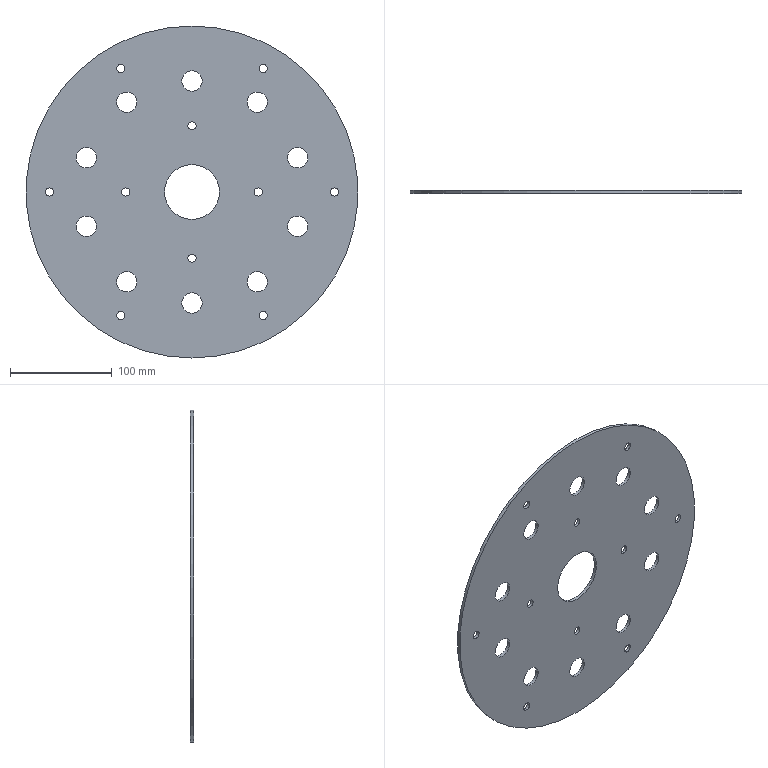Part | STEP file | JBJ-P-1012-03 | 1 solid | 24 faces | box 326 x 3 x 326 mm | volume 232604 mm3 | cylinder 22 | plane 2 | commonest cylinder face diameters 8 x10 20 x10 54 x1 326 x1
STEP:
#1=CARTESIAN_POINT('',(-140.,3.,4.));
#2=VERTEX_POINT('',#1);
#3=CARTESIAN_POINT('',(-140.,3.,0.));
#4=DIRECTION('',(0.,1.,0.));
#5=DIRECTION('',(0.,0.,1.));
#6=AXIS2_PLACEMENT_3D('',#3,#4,#5);
#7=CIRCLE('',#6,4.);
#8=EDGE_CURVE('',#2,#2,#7,.T.);
#9=ORIENTED_EDGE('',*,*,#8,.F.);
#10=EDGE_LOOP('',(#9));
#11=FACE_BOUND('',#10,.T.);
#12=CARTESIAN_POINT('',(-70.,3.,-117.244));
#13=VERTEX_POINT('',#12);
#14=CARTESIAN_POINT('',(-70.,3.,-121.244));
#15=DIRECTION('',(0.,1.,0.));
#16=DIRECTION('',(0.,0.,1.));
#17=AXIS2_PLACEMENT_3D('',#14,#15,#16);
#18=CIRCLE('',#17,4.);
#19=EDGE_CURVE('',#13,#13,#18,.T.);
#20=ORIENTED_EDGE('',*,*,#19,.F.);
#21=EDGE_LOOP('',(#20));
#22=FACE_BOUND('',#21,.T.);
#23=CARTESIAN_POINT('',(70.,3.,-117.244));
#24=VERTEX_POINT('',#23);
#25=CARTESIAN_POINT('',(70.,3.,-121.244));
#26=DIRECTION('',(0.,1.,0.));
#27=DIRECTION('',(0.,0.,1.));
#28=AXIS2_PLACEMENT_3D('',#25,#26,#27);
#29=CIRCLE('',#28,4.);
#30=EDGE_CURVE('',#24,#24,#29,.T.);
#31=ORIENTED_EDGE('',*,*,#30,.F.);
#32=EDGE_LOOP('',(#31));
#33=FACE_BOUND('',#32,.T.);
#34=CARTESIAN_POINT('',(140.,3.,4.));
#35=VERTEX_POINT('',#34);
#36=CARTESIAN_POINT('',(140.,3.,0.));
#37=DIRECTION('',(0.,1.,0.));
#38=DIRECTION('',(0.,0.,1.));
#39=AXIS2_PLACEMENT_3D('',#36,#37,#38);
#40=CIRCLE('',#39,4.);
#41=EDGE_CURVE('',#35,#35,#40,.T.);
#42=ORIENTED_EDGE('',*,*,#41,.F.);
#43=EDGE_LOOP('',(#42));
#44=FACE_BOUND('',#43,.T.);
#45=CARTESIAN_POINT('',(70.,3.,125.244));
#46=VERTEX_POINT('',#45);
#47=CARTESIAN_POINT('',(70.,3.,121.244));
#48=DIRECTION('',(0.,1.,0.));
#49=DIRECTION('',(0.,0.,1.));
#50=AXIS2_PLACEMENT_3D('',#47,#48,#49);
#51=CIRCLE('',#50,4.);
#52=EDGE_CURVE('',#46,#46,#51,.T.);
#53=ORIENTED_EDGE('',*,*,#52,.F.);
#54=EDGE_LOOP('',(#53));
#55=FACE_BOUND('',#54,.T.);
#56=CARTESIAN_POINT('',(-70.,3.,125.244));
#57=VERTEX_POINT('',#56);
#58=CARTESIAN_POINT('',(-70.,3.,121.244));
#59=DIRECTION('',(0.,1.,0.));
#60=DIRECTION('',(0.,0.,1.));
#61=AXIS2_PLACEMENT_3D('',#58,#59,#60);
#62=CIRCLE('',#61,4.);
#63=EDGE_CURVE('',#57,#57,#62,.T.);
#64=ORIENTED_EDGE('',*,*,#63,.F.);
#65=EDGE_LOOP('',(#64));
#66=FACE_BOUND('',#65,.T.);
#67=CARTESIAN_POINT('',(65.,3.,4.));
#68=VERTEX_POINT('',#67);
#69=CARTESIAN_POINT('',(65.,3.,0.));
#70=DIRECTION('',(0.,1.,0.));
#71=DIRECTION('',(0.,0.,1.));
#72=AXIS2_PLACEMENT_3D('',#69,#70,#71);
#73=CIRCLE('',#72,4.);
#74=EDGE_CURVE('',#68,#68,#73,.T.);
#75=ORIENTED_EDGE('',*,*,#74,.F.);
#76=EDGE_LOOP('',(#75));
#77=FACE_BOUND('',#76,.T.);
#78=CARTESIAN_POINT('',(0.,3.,-61.));
#79=VERTEX_POINT('',#78);
#80=CARTESIAN_POINT('',(0.,3.,-65.));
#81=DIRECTION('',(0.,1.,0.));
#82=DIRECTION('',(0.,0.,1.));
#83=AXIS2_PLACEMENT_3D('',#80,#81,#82);
#84=CIRCLE('',#83,4.);
#85=EDGE_CURVE('',#79,#79,#84,.T.);
#86=ORIENTED_EDGE('',*,*,#85,.F.);
#87=EDGE_LOOP('',(#86));
#88=FACE_BOUND('',#87,.T.);
#89=CARTESIAN_POINT('',(-65.,3.,4.));
#90=VERTEX_POINT('',#89);
#91=CARTESIAN_POINT('',(-65.,3.,0.));
#92=DIRECTION('',(0.,1.,0.));
#93=DIRECTION('',(0.,0.,1.));
#94=AXIS2_PLACEMENT_3D('',#91,#92,#93);
#95=CIRCLE('',#94,4.);
#96=EDGE_CURVE('',#90,#90,#95,.T.);
#97=ORIENTED_EDGE('',*,*,#96,.F.);
#98=EDGE_LOOP('',(#97));
#99=FACE_BOUND('',#98,.T.);
#100=CARTESIAN_POINT('',(0.,3.,69.));
#101=VERTEX_POINT('',#100);
#102=CARTESIAN_POINT('',(0.,3.,65.));
#103=DIRECTION('',(0.,1.,0.));
#104=DIRECTION('',(0.,0.,1.));
#105=AXIS2_PLACEMENT_3D('',#102,#103,#104);
#106=CIRCLE('',#105,4.);
#107=EDGE_CURVE('',#101,#101,#106,.T.);
#108=ORIENTED_EDGE('',*,*,#107,.F.);
#109=EDGE_LOOP('',(#108));
#110=FACE_BOUND('',#109,.T.);
#111=CARTESIAN_POINT('',(0.,3.,119.));
#112=VERTEX_POINT('',#111);
#113=CARTESIAN_POINT('',(0.,3.,109.));
#114=DIRECTION('',(0.,1.,0.));
#115=DIRECTION('',(0.,0.,1.));
#116=AXIS2_PLACEMENT_3D('',#113,#114,#115);
#117=CIRCLE('',#116,10.);
#118=EDGE_CURVE('',#112,#112,#117,.T.);
#119=ORIENTED_EDGE('',*,*,#118,.F.);
#120=EDGE_LOOP('',(#119));
#121=FACE_BOUND('',#120,.T.);
#122=CARTESIAN_POINT('',(103.665,3.,43.683));
#123=VERTEX_POINT('',#122);
#124=CARTESIAN_POINT('',(103.665,3.,33.683));
#125=DIRECTION('',(0.,1.,0.));
#126=DIRECTION('',(0.,0.,1.));
#127=AXIS2_PLACEMENT_3D('',#124,#125,#126);
#128=CIRCLE('',#127,10.);
#129=EDGE_CURVE('',#123,#123,#128,.T.);
#130=ORIENTED_EDGE('',*,*,#129,.F.);
#131=EDGE_LOOP('',(#130));
#132=FACE_BOUND('',#131,.T.);
#133=CARTESIAN_POINT('',(64.069,3.,-78.183));
#134=VERTEX_POINT('',#133);
#135=CARTESIAN_POINT('',(64.069,3.,-88.183));
#136=DIRECTION('',(0.,1.,0.));
#137=DIRECTION('',(0.,0.,1.));
#138=AXIS2_PLACEMENT_3D('',#135,#136,#137);
#139=CIRCLE('',#138,10.);
#140=EDGE_CURVE('',#134,#134,#139,.T.);
#141=ORIENTED_EDGE('',*,*,#140,.F.);
#142=EDGE_LOOP('',(#141));
#143=FACE_BOUND('',#142,.T.);
#144=CARTESIAN_POINT('',(-64.069,3.,-78.183));
#145=VERTEX_POINT('',#144);
#146=CARTESIAN_POINT('',(-64.069,3.,-88.183));
#147=DIRECTION('',(0.,1.,0.));
#148=DIRECTION('',(0.,0.,1.));
#149=AXIS2_PLACEMENT_3D('',#146,#147,#148);
#150=CIRCLE('',#149,10.);
#151=EDGE_CURVE('',#145,#145,#150,.T.);
#152=ORIENTED_EDGE('',*,*,#151,.F.);
#153=EDGE_LOOP('',(#152));
#154=FACE_BOUND('',#153,.T.);
#155=CARTESIAN_POINT('',(-103.665,3.,-23.683));
#156=VERTEX_POINT('',#155);
#157=CARTESIAN_POINT('',(-103.665,3.,-33.683));
#158=DIRECTION('',(0.,1.,0.));
#159=DIRECTION('',(0.,0.,1.));
#160=AXIS2_PLACEMENT_3D('',#157,#158,#159);
#161=CIRCLE('',#160,10.);
#162=EDGE_CURVE('',#156,#156,#161,.T.);
#163=ORIENTED_EDGE('',*,*,#162,.F.);
#164=EDGE_LOOP('',(#163));
#165=FACE_BOUND('',#164,.T.);
#166=CARTESIAN_POINT('',(0.,3.,163.));
#167=VERTEX_POINT('',#166);
#168=CARTESIAN_POINT('',(0.,3.,0.));
#169=DIRECTION('',(0.,1.,0.));
#170=DIRECTION('',(0.,0.,1.));
#171=AXIS2_PLACEMENT_3D('',#168,#169,#170);
#172=CIRCLE('',#171,163.);
#173=EDGE_CURVE('',#167,#167,#172,.T.);
#174=ORIENTED_EDGE('',*,*,#173,.T.);
#175=EDGE_LOOP('',(#174));
#176=FACE_OUTER_BOUND('',#175,.T.);
#177=CARTESIAN_POINT('',(0.,3.,27.));
#178=VERTEX_POINT('',#177);
#179=CARTESIAN_POINT('',(0.,3.,0.));
#180=DIRECTION('',(0.,1.,0.));
#181=DIRECTION('',(0.,0.,1.));
#182=AXIS2_PLACEMENT_3D('',#179,#180,#181);
#183=CIRCLE('',#182,27.);
#184=EDGE_CURVE('',#178,#178,#183,.T.);
#185=ORIENTED_EDGE('',*,*,#184,.F.);
#186=EDGE_LOOP('',(#185));
#187=FACE_BOUND('',#186,.T.);
#188=CARTESIAN_POINT('',(-103.665,3.,43.683));
#189=VERTEX_POINT('',#188);
#190=CARTESIAN_POINT('',(-103.665,3.,33.683));
#191=DIRECTION('',(0.,1.,0.));
#192=DIRECTION('',(0.,0.,1.));
#193=AXIS2_PLACEMENT_3D('',#190,#191,#192);
#194=CIRCLE('',#193,10.);
#195=EDGE_CURVE('',#189,#189,#194,.T.);
#196=ORIENTED_EDGE('',*,*,#195,.F.);
#197=EDGE_LOOP('',(#196));
#198=FACE_BOUND('',#197,.T.);
#199=CARTESIAN_POINT('',(0.,3.,-99.));
#200=VERTEX_POINT('',#199);
#201=CARTESIAN_POINT('',(0.,3.,-109.));
#202=DIRECTION('',(0.,1.,0.));
#203=DIRECTION('',(0.,0.,1.));
#204=AXIS2_PLACEMENT_3D('',#201,#202,#203);
#205=CIRCLE('',#204,10.);
#206=EDGE_CURVE('',#200,#200,#205,.T.);
#207=ORIENTED_EDGE('',*,*,#206,.F.);
#208=EDGE_LOOP('',(#207));
#209=FACE_BOUND('',#208,.T.);
#210=CARTESIAN_POINT('',(103.665,3.,-23.683));
#211=VERTEX_POINT('',#210);
#212=CARTESIAN_POINT('',(103.665,3.,-33.683));
#213=DIRECTION('',(0.,1.,0.));
#214=DIRECTION('',(0.,0.,1.));
#215=AXIS2_PLACEMENT_3D('',#212,#213,#214);
#216=CIRCLE('',#215,10.);
#217=EDGE_CURVE('',#211,#211,#216,.T.);
#218=ORIENTED_EDGE('',*,*,#217,.F.);
#219=EDGE_LOOP('',(#218));
#220=FACE_BOUND('',#219,.T.);
#221=CARTESIAN_POINT('',(64.069,3.,98.183));
#222=VERTEX_POINT('',#221);
#223=CARTESIAN_POINT('',(64.069,3.,88.183));
#224=DIRECTION('',(0.,1.,0.));
#225=DIRECTION('',(0.,0.,1.));
#226=AXIS2_PLACEMENT_3D('',#223,#224,#225);
#227=CIRCLE('',#226,10.);
#228=EDGE_CURVE('',#222,#222,#227,.T.);
#229=ORIENTED_EDGE('',*,*,#228,.F.);
#230=EDGE_LOOP('',(#229));
#231=FACE_BOUND('',#230,.T.);
#232=CARTESIAN_POINT('',(-64.069,3.,98.183));
#233=VERTEX_POINT('',#232);
#234=CARTESIAN_POINT('',(-64.069,3.,88.183));
#235=DIRECTION('',(0.,1.,0.));
#236=DIRECTION('',(0.,0.,1.));
#237=AXIS2_PLACEMENT_3D('',#234,#235,#236);
#238=CIRCLE('',#237,10.);
#239=EDGE_CURVE('',#233,#233,#238,.T.);
#240=ORIENTED_EDGE('',*,*,#239,.F.);
#241=EDGE_LOOP('',(#240));
#242=FACE_BOUND('',#241,.T.);
#243=CARTESIAN_POINT('',(0.,3.,0.));
#244=DIRECTION('',(0.,1.,0.));
#245=DIRECTION('',(0.,0.,1.));
#246=AXIS2_PLACEMENT_3D('',#243,#244,#245);
#247=PLANE('',#246);
#248=ADVANCED_FACE('',(#11,#22,#33,#44,#55,#66,#77,#88,#99,#110,#121,#132,#143,#154,#165,#176,#187,#198,#209,#220,#231,#242),#247,.T.);
#249=CARTESIAN_POINT('',(-140.,0.,4.));
#250=VERTEX_POINT('',#249);
#251=CARTESIAN_POINT('',(-140.,0.,0.));
#252=DIRECTION('',(0.,1.,0.));
#253=DIRECTION('',(0.,0.,1.));
#254=AXIS2_PLACEMENT_3D('',#251,#252,#253);
#255=CIRCLE('',#254,4.);
#256=EDGE_CURVE('',#250,#250,#255,.T.);
#257=ORIENTED_EDGE('',*,*,#256,.T.);
#258=EDGE_LOOP('',(#257));
#259=FACE_BOUND('',#258,.T.);
#260=CARTESIAN_POINT('',(-70.,0.,-117.244));
#261=VERTEX_POINT('',#260);
#262=CARTESIAN_POINT('',(-70.,0.,-121.244));
#263=DIRECTION('',(0.,1.,0.));
#264=DIRECTION('',(0.,0.,1.));
#265=AXIS2_PLACEMENT_3D('',#262,#263,#264);
#266=CIRCLE('',#265,4.);
#267=EDGE_CURVE('',#261,#261,#266,.T.);
#268=ORIENTED_EDGE('',*,*,#267,.T.);
#269=EDGE_LOOP('',(#268));
#270=FACE_BOUND('',#269,.T.);
#271=CARTESIAN_POINT('',(70.,0.,-117.244));
#272=VERTEX_POINT('',#271);
#273=CARTESIAN_POINT('',(70.,0.,-121.244));
#274=DIRECTION('',(0.,1.,0.));
#275=DIRECTION('',(0.,0.,1.));
#276=AXIS2_PLACEMENT_3D('',#273,#274,#275);
#277=CIRCLE('',#276,4.);
#278=EDGE_CURVE('',#272,#272,#277,.T.);
#279=ORIENTED_EDGE('',*,*,#278,.T.);
#280=EDGE_LOOP('',(#279));
#281=FACE_BOUND('',#280,.T.);
#282=CARTESIAN_POINT('',(140.,0.,4.));
#283=VERTEX_POINT('',#282);
#284=CARTESIAN_POINT('',(140.,0.,0.));
#285=DIRECTION('',(0.,1.,0.));
#286=DIRECTION('',(0.,0.,1.));
#287=AXIS2_PLACEMENT_3D('',#284,#285,#286);
#288=CIRCLE('',#287,4.);
#289=EDGE_CURVE('',#283,#283,#288,.T.);
#290=ORIENTED_EDGE('',*,*,#289,.T.);
#291=EDGE_LOOP('',(#290));
#292=FACE_BOUND('',#291,.T.);
#293=CARTESIAN_POINT('',(70.,0.,125.244));
#294=VERTEX_POINT('',#293);
#295=CARTESIAN_POINT('',(70.,0.,121.244));
#296=DIRECTION('',(0.,1.,0.));
#297=DIRECTION('',(0.,0.,1.));
#298=AXIS2_PLACEMENT_3D('',#295,#296,#297);
#299=CIRCLE('',#298,4.);
#300=EDGE_CURVE('',#294,#294,#299,.T.);
#301=ORIENTED_EDGE('',*,*,#300,.T.);
#302=EDGE_LOOP('',(#301));
#303=FACE_BOUND('',#302,.T.);
#304=CARTESIAN_POINT('',(-70.,0.,125.244));
#305=VERTEX_POINT('',#304);
#306=CARTESIAN_POINT('',(-70.,0.,121.244));
#307=DIRECTION('',(0.,1.,0.));
#308=DIRECTION('',(0.,0.,1.));
#309=AXIS2_PLACEMENT_3D('',#306,#307,#308);
#310=CIRCLE('',#309,4.);
#311=EDGE_CURVE('',#305,#305,#310,.T.);
#312=ORIENTED_EDGE('',*,*,#311,.T.);
#313=EDGE_LOOP('',(#312));
#314=FACE_BOUND('',#313,.T.);
#315=CARTESIAN_POINT('',(65.,0.,4.));
#316=VERTEX_POINT('',#315);
#317=CARTESIAN_POINT('',(65.,0.,0.));
#318=DIRECTION('',(0.,1.,0.));
#319=DIRECTION('',(0.,0.,1.));
#320=AXIS2_PLACEMENT_3D('',#317,#318,#319);
#321=CIRCLE('',#320,4.);
#322=EDGE_CURVE('',#316,#316,#321,.T.);
#323=ORIENTED_EDGE('',*,*,#322,.T.);
#324=EDGE_LOOP('',(#323));
#325=FACE_BOUND('',#324,.T.);
#326=CARTESIAN_POINT('',(0.,0.,-61.));
#327=VERTEX_POINT('',#326);
#328=CARTESIAN_POINT('',(0.,0.,-65.));
#329=DIRECTION('',(0.,1.,0.));
#330=DIRECTION('',(0.,0.,1.));
#331=AXIS2_PLACEMENT_3D('',#328,#329,#330);
#332=CIRCLE('',#331,4.);
#333=EDGE_CURVE('',#327,#327,#332,.T.);
#334=ORIENTED_EDGE('',*,*,#333,.T.);
#335=EDGE_LOOP('',(#334));
#336=FACE_BOUND('',#335,.T.);
#337=CARTESIAN_POINT('',(-65.,0.,4.));
#338=VERTEX_POINT('',#337);
#339=CARTESIAN_POINT('',(-65.,0.,0.));
#340=DIRECTION('',(0.,1.,0.));
#341=DIRECTION('',(0.,0.,1.));
#342=AXIS2_PLACEMENT_3D('',#339,#340,#341);
#343=CIRCLE('',#342,4.);
#344=EDGE_CURVE('',#338,#338,#343,.T.);
#345=ORIENTED_EDGE('',*,*,#344,.T.);
#346=EDGE_LOOP('',(#345));
#347=FACE_BOUND('',#346,.T.);
#348=CARTESIAN_POINT('',(0.,0.,69.));
#349=VERTEX_POINT('',#348);
#350=CARTESIAN_POINT('',(0.,0.,65.));
#351=DIRECTION('',(0.,1.,0.));
#352=DIRECTION('',(0.,0.,1.));
#353=AXIS2_PLACEMENT_3D('',#350,#351,#352);
#354=CIRCLE('',#353,4.);
#355=EDGE_CURVE('',#349,#349,#354,.T.);
#356=ORIENTED_EDGE('',*,*,#355,.T.);
#357=EDGE_LOOP('',(#356));
#358=FACE_BOUND('',#357,.T.);
#359=CARTESIAN_POINT('',(0.,0.,163.));
#360=VERTEX_POINT('',#359);
#361=CARTESIAN_POINT('',(0.,0.,0.));
#362=DIRECTION('',(0.,1.,0.));
#363=DIRECTION('',(0.,0.,1.));
#364=AXIS2_PLACEMENT_3D('',#361,#362,#363);
#365=CIRCLE('',#364,163.);
#366=EDGE_CURVE('',#360,#360,#365,.T.);
#367=ORIENTED_EDGE('',*,*,#366,.F.);
#368=EDGE_LOOP('',(#367));
#369=FACE_OUTER_BOUND('',#368,.T.);
#370=CARTESIAN_POINT('',(0.,0.,27.));
#371=VERTEX_POINT('',#370);
#372=CARTESIAN_POINT('',(0.,0.,0.));
#373=DIRECTION('',(0.,1.,0.));
#374=DIRECTION('',(0.,0.,1.));
#375=AXIS2_PLACEMENT_3D('',#372,#373,#374);
#376=CIRCLE('',#375,27.);
#377=EDGE_CURVE('',#371,#371,#376,.T.);
#378=ORIENTED_EDGE('',*,*,#377,.T.);
#379=EDGE_LOOP('',(#378));
#380=FACE_BOUND('',#379,.T.);
#381=CARTESIAN_POINT('',(-103.665,0.,-23.683));
#382=VERTEX_POINT('',#381);
#383=CARTESIAN_POINT('',(-103.665,0.,-33.683));
#384=DIRECTION('',(0.,1.,0.));
#385=DIRECTION('',(0.,0.,1.));
#386=AXIS2_PLACEMENT_3D('',#383,#384,#385);
#387=CIRCLE('',#386,10.);
#388=EDGE_CURVE('',#382,#382,#387,.T.);
#389=ORIENTED_EDGE('',*,*,#388,.T.);
#390=EDGE_LOOP('',(#389));
#391=FACE_BOUND('',#390,.T.);
#392=CARTESIAN_POINT('',(-103.665,0.,43.683));
#393=VERTEX_POINT('',#392);
#394=CARTESIAN_POINT('',(-103.665,0.,33.683));
#395=DIRECTION('',(0.,1.,0.));
#396=DIRECTION('',(0.,0.,1.));
#397=AXIS2_PLACEMENT_3D('',#394,#395,#396);
#398=CIRCLE('',#397,10.);
#399=EDGE_CURVE('',#393,#393,#398,.T.);
#400=ORIENTED_EDGE('',*,*,#399,.T.);
#401=EDGE_LOOP('',(#400));
#402=FACE_BOUND('',#401,.T.);
#403=CARTESIAN_POINT('',(-64.069,0.,-78.183));
#404=VERTEX_POINT('',#403);
#405=CARTESIAN_POINT('',(-64.069,0.,-88.183));
#406=DIRECTION('',(0.,1.,0.));
#407=DIRECTION('',(0.,0.,1.));
#408=AXIS2_PLACEMENT_3D('',#405,#406,#407);
#409=CIRCLE('',#408,10.);
#410=EDGE_CURVE('',#404,#404,#409,.T.);
#411=ORIENTED_EDGE('',*,*,#410,.T.);
#412=EDGE_LOOP('',(#411));
#413=FACE_BOUND('',#412,.T.);
#414=CARTESIAN_POINT('',(0.,0.,-99.));
#415=VERTEX_POINT('',#414);
#416=CARTESIAN_POINT('',(0.,0.,-109.));
#417=DIRECTION('',(0.,1.,0.));
#418=DIRECTION('',(0.,0.,1.));
#419=AXIS2_PLACEMENT_3D('',#416,#417,#418);
#420=CIRCLE('',#419,10.);
#421=EDGE_CURVE('',#415,#415,#420,.T.);
#422=ORIENTED_EDGE('',*,*,#421,.T.);
#423=EDGE_LOOP('',(#422));
#424=FACE_BOUND('',#423,.T.);
#425=CARTESIAN_POINT('',(64.069,0.,-78.183));
#426=VERTEX_POINT('',#425);
#427=CARTESIAN_POINT('',(64.069,0.,-88.183));
#428=DIRECTION('',(0.,1.,0.));
#429=DIRECTION('',(0.,0.,1.));
#430=AXIS2_PLACEMENT_3D('',#427,#428,#429);
#431=CIRCLE('',#430,10.);
#432=EDGE_CURVE('',#426,#426,#431,.T.);
#433=ORIENTED_EDGE('',*,*,#432,.T.);
#434=EDGE_LOOP('',(#433));
#435=FACE_BOUND('',#434,.T.);
#436=CARTESIAN_POINT('',(103.665,0.,-23.683));
#437=VERTEX_POINT('',#436);
#438=CARTESIAN_POINT('',(103.665,0.,-33.683));
#439=DIRECTION('',(0.,1.,0.));
#440=DIRECTION('',(0.,0.,1.));
#441=AXIS2_PLACEMENT_3D('',#438,#439,#440);
#442=CIRCLE('',#441,10.);
#443=EDGE_CURVE('',#437,#437,#442,.T.);
#444=ORIENTED_EDGE('',*,*,#443,.T.);
#445=EDGE_LOOP('',(#444));
#446=FACE_BOUND('',#445,.T.);
#447=CARTESIAN_POINT('',(103.665,0.,43.683));
#448=VERTEX_POINT('',#447);
#449=CARTESIAN_POINT('',(103.665,0.,33.683));
#450=DIRECTION('',(0.,1.,0.));
#451=DIRECTION('',(0.,0.,1.));
#452=AXIS2_PLACEMENT_3D('',#449,#450,#451);
#453=CIRCLE('',#452,10.);
#454=EDGE_CURVE('',#448,#448,#453,.T.);
#455=ORIENTED_EDGE('',*,*,#454,.T.);
#456=EDGE_LOOP('',(#455));
#457=FACE_BOUND('',#456,.T.);
#458=CARTESIAN_POINT('',(64.069,0.,98.183));
#459=VERTEX_POINT('',#458);
#460=CARTESIAN_POINT('',(64.069,0.,88.183));
#461=DIRECTION('',(0.,1.,0.));
#462=DIRECTION('',(0.,0.,1.));
#463=AXIS2_PLACEMENT_3D('',#460,#461,#462);
#464=CIRCLE('',#463,10.);
#465=EDGE_CURVE('',#459,#459,#464,.T.);
#466=ORIENTED_EDGE('',*,*,#465,.T.);
#467=EDGE_LOOP('',(#466));
#468=FACE_BOUND('',#467,.T.);
#469=CARTESIAN_POINT('',(0.,0.,119.));
#470=VERTEX_POINT('',#469);
#471=CARTESIAN_POINT('',(0.,0.,109.));
#472=DIRECTION('',(0.,1.,0.));
#473=DIRECTION('',(0.,0.,1.));
#474=AXIS2_PLACEMENT_3D('',#471,#472,#473);
#475=CIRCLE('',#474,10.);
#476=EDGE_CURVE('',#470,#470,#475,.T.);
#477=ORIENTED_EDGE('',*,*,#476,.T.);
#478=EDGE_LOOP('',(#477));
#479=FACE_BOUND('',#478,.T.);
#480=CARTESIAN_POINT('',(-64.069,0.,98.183));
#481=VERTEX_POINT('',#480);
#482=CARTESIAN_POINT('',(-64.069,0.,88.183));
#483=DIRECTION('',(0.,1.,0.));
#484=DIRECTION('',(0.,0.,1.));
#485=AXIS2_PLACEMENT_3D('',#482,#483,#484);
#486=CIRCLE('',#485,10.);
#487=EDGE_CURVE('',#481,#481,#486,.T.);
#488=ORIENTED_EDGE('',*,*,#487,.T.);
#489=EDGE_LOOP('',(#488));
#490=FACE_BOUND('',#489,.T.);
#491=CARTESIAN_POINT('',(0.,0.,0.));
#492=DIRECTION('',(0.,1.,0.));
#493=DIRECTION('',(0.,0.,1.));
#494=AXIS2_PLACEMENT_3D('',#491,#492,#493);
#495=PLANE('',#494);
#496=ADVANCED_FACE('',(#259,#270,#281,#292,#303,#314,#325,#336,#347,#358,#369,#380,#391,#402,#413,#424,#435,#446,#457,#468,#479,#490),#495,.F.);
#497=ORIENTED_EDGE('',*,*,#173,.F.);
#498=EDGE_LOOP('',(#497));
#499=FACE_OUTER_BOUND('',#498,.T.);
#500=ORIENTED_EDGE('',*,*,#366,.T.);
#501=EDGE_LOOP('',(#500));
#502=FACE_OUTER_BOUND('',#501,.T.);
#503=CARTESIAN_POINT('',(0.,3.,0.));
#504=DIRECTION('',(0.,-1.,0.));
#505=DIRECTION('',(0.,0.,-1.));
#506=AXIS2_PLACEMENT_3D('',#503,#504,#505);
#507=CYLINDRICAL_SURFACE('',#506,163.);
#508=ADVANCED_FACE('',(#499,#502),#507,.T.);
#509=ORIENTED_EDGE('',*,*,#184,.T.);
#510=EDGE_LOOP('',(#509));
#511=FACE_OUTER_BOUND('',#510,.T.);
#512=ORIENTED_EDGE('',*,*,#377,.F.);
#513=EDGE_LOOP('',(#512));
#514=FACE_OUTER_BOUND('',#513,.T.);
#515=CARTESIAN_POINT('',(0.,3.,0.));
#516=DIRECTION('',(0.,-1.,0.));
#517=DIRECTION('',(0.,0.,-1.));
#518=AXIS2_PLACEMENT_3D('',#515,#516,#517);
#519=CYLINDRICAL_SURFACE('',#518,27.);
#520=ADVANCED_FACE('',(#511,#514),#519,.F.);
#521=ORIENTED_EDGE('',*,*,#162,.T.);
#522=EDGE_LOOP('',(#521));
#523=FACE_OUTER_BOUND('',#522,.T.);
#524=ORIENTED_EDGE('',*,*,#388,.F.);
#525=EDGE_LOOP('',(#524));
#526=FACE_OUTER_BOUND('',#525,.T.);
#527=CARTESIAN_POINT('',(-103.665,3.,-33.683));
#528=DIRECTION('',(0.,-1.,0.));
#529=DIRECTION('',(0.,0.,-1.));
#530=AXIS2_PLACEMENT_3D('',#527,#528,#529);
#531=CYLINDRICAL_SURFACE('',#530,10.);
#532=ADVANCED_FACE('',(#523,#526),#531,.F.);
#533=ORIENTED_EDGE('',*,*,#195,.T.);
#534=EDGE_LOOP('',(#533));
#535=FACE_OUTER_BOUND('',#534,.T.);
#536=ORIENTED_EDGE('',*,*,#399,.F.);
#537=EDGE_LOOP('',(#536));
#538=FACE_OUTER_BOUND('',#537,.T.);
#539=CARTESIAN_POINT('',(-103.665,3.,33.683));
#540=DIRECTION('',(0.,-1.,0.));
#541=DIRECTION('',(0.,0.,-1.));
#542=AXIS2_PLACEMENT_3D('',#539,#540,#541);
#543=CYLINDRICAL_SURFACE('',#542,10.);
#544=ADVANCED_FACE('',(#535,#538),#543,.F.);
#545=ORIENTED_EDGE('',*,*,#151,.T.);
#546=EDGE_LOOP('',(#545));
#547=FACE_OUTER_BOUND('',#546,.T.);
#548=ORIENTED_EDGE('',*,*,#410,.F.);
#549=EDGE_LOOP('',(#548));
#550=FACE_OUTER_BOUND('',#549,.T.);
#551=CARTESIAN_POINT('',(-64.069,3.,-88.183));
#552=DIRECTION('',(0.,-1.,0.));
#553=DIRECTION('',(0.,0.,-1.));
#554=AXIS2_PLACEMENT_3D('',#551,#552,#553);
#555=CYLINDRICAL_SURFACE('',#554,10.);
#556=ADVANCED_FACE('',(#547,#550),#555,.F.);
#557=ORIENTED_EDGE('',*,*,#206,.T.);
#558=EDGE_LOOP('',(#557));
#559=FACE_OUTER_BOUND('',#558,.T.);
#560=ORIENTED_EDGE('',*,*,#421,.F.);
#561=EDGE_LOOP('',(#560));
#562=FACE_OUTER_BOUND('',#561,.T.);
#563=CARTESIAN_POINT('',(0.,3.,-109.));
#564=DIRECTION('',(0.,-1.,0.));
#565=DIRECTION('',(0.,0.,-1.));
#566=AXIS2_PLACEMENT_3D('',#563,#564,#565);
#567=CYLINDRICAL_SURFACE('',#566,10.);
#568=ADVANCED_FACE('',(#559,#562),#567,.F.);
#569=ORIENTED_EDGE('',*,*,#140,.T.);
#570=EDGE_LOOP('',(#569));
#571=FACE_OUTER_BOUND('',#570,.T.);
#572=ORIENTED_EDGE('',*,*,#432,.F.);
#573=EDGE_LOOP('',(#572));
#574=FACE_OUTER_BOUND('',#573,.T.);
#575=CARTESIAN_POINT('',(64.069,3.,-88.183));
#576=DIRECTION('',(0.,-1.,0.));
#577=DIRECTION('',(0.,0.,-1.));
#578=AXIS2_PLACEMENT_3D('',#575,#576,#577);
#579=CYLINDRICAL_SURFACE('',#578,10.);
#580=ADVANCED_FACE('',(#571,#574),#579,.F.);
#581=ORIENTED_EDGE('',*,*,#217,.T.);
#582=EDGE_LOOP('',(#581));
#583=FACE_OUTER_BOUND('',#582,.T.);
#584=ORIENTED_EDGE('',*,*,#443,.F.);
#585=EDGE_LOOP('',(#584));
#586=FACE_OUTER_BOUND('',#585,.T.);
#587=CARTESIAN_POINT('',(103.665,3.,-33.683));
#588=DIRECTION('',(0.,-1.,0.));
#589=DIRECTION('',(0.,0.,-1.));
#590=AXIS2_PLACEMENT_3D('',#587,#588,#589);
#591=CYLINDRICAL_SURFACE('',#590,10.);
#592=ADVANCED_FACE('',(#583,#586),#591,.F.);
#593=ORIENTED_EDGE('',*,*,#129,.T.);
#594=EDGE_LOOP('',(#593));
#595=FACE_OUTER_BOUND('',#594,.T.);
#596=ORIENTED_EDGE('',*,*,#454,.F.);
#597=EDGE_LOOP('',(#596));
#598=FACE_OUTER_BOUND('',#597,.T.);
#599=CARTESIAN_POINT('',(103.665,3.,33.683));
#600=DIRECTION('',(0.,-1.,0.));
#601=DIRECTION('',(0.,0.,-1.));
#602=AXIS2_PLACEMENT_3D('',#599,#600,#601);
#603=CYLINDRICAL_SURFACE('',#602,10.);
#604=ADVANCED_FACE('',(#595,#598),#603,.F.);
#605=ORIENTED_EDGE('',*,*,#228,.T.);
#606=EDGE_LOOP('',(#605));
#607=FACE_OUTER_BOUND('',#606,.T.);
#608=ORIENTED_EDGE('',*,*,#465,.F.);
#609=EDGE_LOOP('',(#608));
#610=FACE_OUTER_BOUND('',#609,.T.);
#611=CARTESIAN_POINT('',(64.069,3.,88.183));
#612=DIRECTION('',(0.,-1.,0.));
#613=DIRECTION('',(0.,0.,-1.));
#614=AXIS2_PLACEMENT_3D('',#611,#612,#613);
#615=CYLINDRICAL_SURFACE('',#614,10.);
#616=ADVANCED_FACE('',(#607,#610),#615,.F.);
#617=ORIENTED_EDGE('',*,*,#118,.T.);
#618=EDGE_LOOP('',(#617));
#619=FACE_OUTER_BOUND('',#618,.T.);
#620=ORIENTED_EDGE('',*,*,#476,.F.);
#621=EDGE_LOOP('',(#620));
#622=FACE_OUTER_BOUND('',#621,.T.);
#623=CARTESIAN_POINT('',(0.,3.,109.));
#624=DIRECTION('',(0.,-1.,0.));
#625=DIRECTION('',(0.,0.,-1.));
#626=AXIS2_PLACEMENT_3D('',#623,#624,#625);
#627=CYLINDRICAL_SURFACE('',#626,10.);
#628=ADVANCED_FACE('',(#619,#622),#627,.F.);
#629=ORIENTED_EDGE('',*,*,#239,.T.);
#630=EDGE_LOOP('',(#629));
#631=FACE_OUTER_BOUND('',#630,.T.);
#632=ORIENTED_EDGE('',*,*,#487,.F.);
#633=EDGE_LOOP('',(#632));
#634=FACE_OUTER_BOUND('',#633,.T.);
#635=CARTESIAN_POINT('',(-64.069,3.,88.183));
#636=DIRECTION('',(0.,-1.,0.));
#637=DIRECTION('',(0.,0.,-1.));
#638=AXIS2_PLACEMENT_3D('',#635,#636,#637);
#639=CYLINDRICAL_SURFACE('',#638,10.);
#640=ADVANCED_FACE('',(#631,#634),#639,.F.);
#641=ORIENTED_EDGE('',*,*,#355,.F.);
#642=EDGE_LOOP('',(#641));
#643=FACE_OUTER_BOUND('',#642,.T.);
#644=ORIENTED_EDGE('',*,*,#107,.T.);
#645=EDGE_LOOP('',(#644));
#646=FACE_OUTER_BOUND('',#645,.T.);
#647=CARTESIAN_POINT('',(0.,3.,65.));
#648=DIRECTION('',(0.,1.,0.));
#649=DIRECTION('',(0.,0.,1.));
#650=AXIS2_PLACEMENT_3D('',#647,#648,#649);
#651=CYLINDRICAL_SURFACE('',#650,4.);
#652=ADVANCED_FACE('',(#643,#646),#651,.F.);
#653=ORIENTED_EDGE('',*,*,#344,.F.);
#654=EDGE_LOOP('',(#653));
#655=FACE_OUTER_BOUND('',#654,.T.);
#656=ORIENTED_EDGE('',*,*,#96,.T.);
#657=EDGE_LOOP('',(#656));
#658=FACE_OUTER_BOUND('',#657,.T.);
#659=CARTESIAN_POINT('',(-65.,3.,0.));
#660=DIRECTION('',(0.,1.,0.));
#661=DIRECTION('',(0.,0.,1.));
#662=AXIS2_PLACEMENT_3D('',#659,#660,#661);
#663=CYLINDRICAL_SURFACE('',#662,4.);
#664=ADVANCED_FACE('',(#655,#658),#663,.F.);
#665=ORIENTED_EDGE('',*,*,#333,.F.);
#666=EDGE_LOOP('',(#665));
#667=FACE_OUTER_BOUND('',#666,.T.);
#668=ORIENTED_EDGE('',*,*,#85,.T.);
#669=EDGE_LOOP('',(#668));
#670=FACE_OUTER_BOUND('',#669,.T.);
#671=CARTESIAN_POINT('',(0.,3.,-65.));
#672=DIRECTION('',(0.,1.,0.));
#673=DIRECTION('',(0.,0.,1.));
#674=AXIS2_PLACEMENT_3D('',#671,#672,#673);
#675=CYLINDRICAL_SURFACE('',#674,4.);
#676=ADVANCED_FACE('',(#667,#670),#675,.F.);
#677=ORIENTED_EDGE('',*,*,#322,.F.);
#678=EDGE_LOOP('',(#677));
#679=FACE_OUTER_BOUND('',#678,.T.);
#680=ORIENTED_EDGE('',*,*,#74,.T.);
#681=EDGE_LOOP('',(#680));
#682=FACE_OUTER_BOUND('',#681,.T.);
#683=CARTESIAN_POINT('',(65.,3.,0.));
#684=DIRECTION('',(0.,1.,0.));
#685=DIRECTION('',(0.,0.,1.));
#686=AXIS2_PLACEMENT_3D('',#683,#684,#685);
#687=CYLINDRICAL_SURFACE('',#686,4.);
#688=ADVANCED_FACE('',(#679,#682),#687,.F.);
#689=ORIENTED_EDGE('',*,*,#311,.F.);
#690=EDGE_LOOP('',(#689));
#691=FACE_OUTER_BOUND('',#690,.T.);
#692=ORIENTED_EDGE('',*,*,#63,.T.);
#693=EDGE_LOOP('',(#692));
#694=FACE_OUTER_BOUND('',#693,.T.);
#695=CARTESIAN_POINT('',(-70.,3.,121.244));
#696=DIRECTION('',(0.,1.,0.));
#697=DIRECTION('',(0.,0.,1.));
#698=AXIS2_PLACEMENT_3D('',#695,#696,#697);
#699=CYLINDRICAL_SURFACE('',#698,4.);
#700=ADVANCED_FACE('',(#691,#694),#699,.F.);
#701=ORIENTED_EDGE('',*,*,#300,.F.);
#702=EDGE_LOOP('',(#701));
#703=FACE_OUTER_BOUND('',#702,.T.);
#704=ORIENTED_EDGE('',*,*,#52,.T.);
#705=EDGE_LOOP('',(#704));
#706=FACE_OUTER_BOUND('',#705,.T.);
#707=CARTESIAN_POINT('',(70.,3.,121.244));
#708=DIRECTION('',(0.,1.,0.));
#709=DIRECTION('',(0.,0.,1.));
#710=AXIS2_PLACEMENT_3D('',#707,#708,#709);
#711=CYLINDRICAL_SURFACE('',#710,4.);
#712=ADVANCED_FACE('',(#703,#706),#711,.F.);
#713=ORIENTED_EDGE('',*,*,#289,.F.);
#714=EDGE_LOOP('',(#713));
#715=FACE_OUTER_BOUND('',#714,.T.);
#716=ORIENTED_EDGE('',*,*,#41,.T.);
#717=EDGE_LOOP('',(#716));
#718=FACE_OUTER_BOUND('',#717,.T.);
#719=CARTESIAN_POINT('',(140.,3.,0.));
#720=DIRECTION('',(0.,1.,0.));
#721=DIRECTION('',(0.,0.,1.));
#722=AXIS2_PLACEMENT_3D('',#719,#720,#721);
#723=CYLINDRICAL_SURFACE('',#722,4.);
#724=ADVANCED_FACE('',(#715,#718),#723,.F.);
#725=ORIENTED_EDGE('',*,*,#278,.F.);
#726=EDGE_LOOP('',(#725));
#727=FACE_OUTER_BOUND('',#726,.T.);
#728=ORIENTED_EDGE('',*,*,#30,.T.);
#729=EDGE_LOOP('',(#728));
#730=FACE_OUTER_BOUND('',#729,.T.);
#731=CARTESIAN_POINT('',(70.,3.,-121.244));
#732=DIRECTION('',(0.,1.,0.));
#733=DIRECTION('',(0.,0.,1.));
#734=AXIS2_PLACEMENT_3D('',#731,#732,#733);
#735=CYLINDRICAL_SURFACE('',#734,4.);
#736=ADVANCED_FACE('',(#727,#730),#735,.F.);
#737=ORIENTED_EDGE('',*,*,#267,.F.);
#738=EDGE_LOOP('',(#737));
#739=FACE_OUTER_BOUND('',#738,.T.);
#740=ORIENTED_EDGE('',*,*,#19,.T.);
#741=EDGE_LOOP('',(#740));
#742=FACE_OUTER_BOUND('',#741,.T.);
#743=CARTESIAN_POINT('',(-70.,3.,-121.244));
#744=DIRECTION('',(0.,1.,0.));
#745=DIRECTION('',(0.,0.,1.));
#746=AXIS2_PLACEMENT_3D('',#743,#744,#745);
#747=CYLINDRICAL_SURFACE('',#746,4.);
#748=ADVANCED_FACE('',(#739,#742),#747,.F.);
#749=ORIENTED_EDGE('',*,*,#256,.F.);
#750=EDGE_LOOP('',(#749));
#751=FACE_OUTER_BOUND('',#750,.T.);
#752=ORIENTED_EDGE('',*,*,#8,.T.);
#753=EDGE_LOOP('',(#752));
#754=FACE_OUTER_BOUND('',#753,.T.);
#755=CARTESIAN_POINT('',(-140.,3.,0.));
#756=DIRECTION('',(0.,1.,0.));
#757=DIRECTION('',(0.,0.,1.));
#758=AXIS2_PLACEMENT_3D('',#755,#756,#757);
#759=CYLINDRICAL_SURFACE('',#758,4.);
#760=ADVANCED_FACE('',(#751,#754),#759,.F.);
#761=CLOSED_SHELL('',(#248,#496,#508,#520,#532,#544,#556,#568,#580,#592,#604,#616,#628,#640,#652,#664,#676,#688,#700,#712,#724,#736,#748,#760));
#762=MANIFOLD_SOLID_BREP('',#761);
#763=CARTESIAN_POINT('',(0.,0.,0.));
#764=DIRECTION('',(0.,0.,1.));
#765=DIRECTION('',(1.,0.,0.));
#766=AXIS2_PLACEMENT_3D('',#763,#764,#765);
#767=(LENGTH_UNIT()NAMED_UNIT(*)SI_UNIT(.MILLI.,.METRE.));
#768=UNCERTAINTY_MEASURE_WITH_UNIT(LENGTH_MEASURE(0.00001),#767,'','');
#769=(NAMED_UNIT(*)PLANE_ANGLE_UNIT()SI_UNIT($,.RADIAN.));
#770=(NAMED_UNIT(*)SI_UNIT($,.STERADIAN.)SOLID_ANGLE_UNIT());
#771=(GEOMETRIC_REPRESENTATION_CONTEXT(3)GLOBAL_UNCERTAINTY_ASSIGNED_CONTEXT((#768))GLOBAL_UNIT_ASSIGNED_CONTEXT((#767,#769,#770))REPRESENTATION_CONTEXT('',''));
#772=ADVANCED_BREP_SHAPE_REPRESENTATION('',(#762,#766),#771);